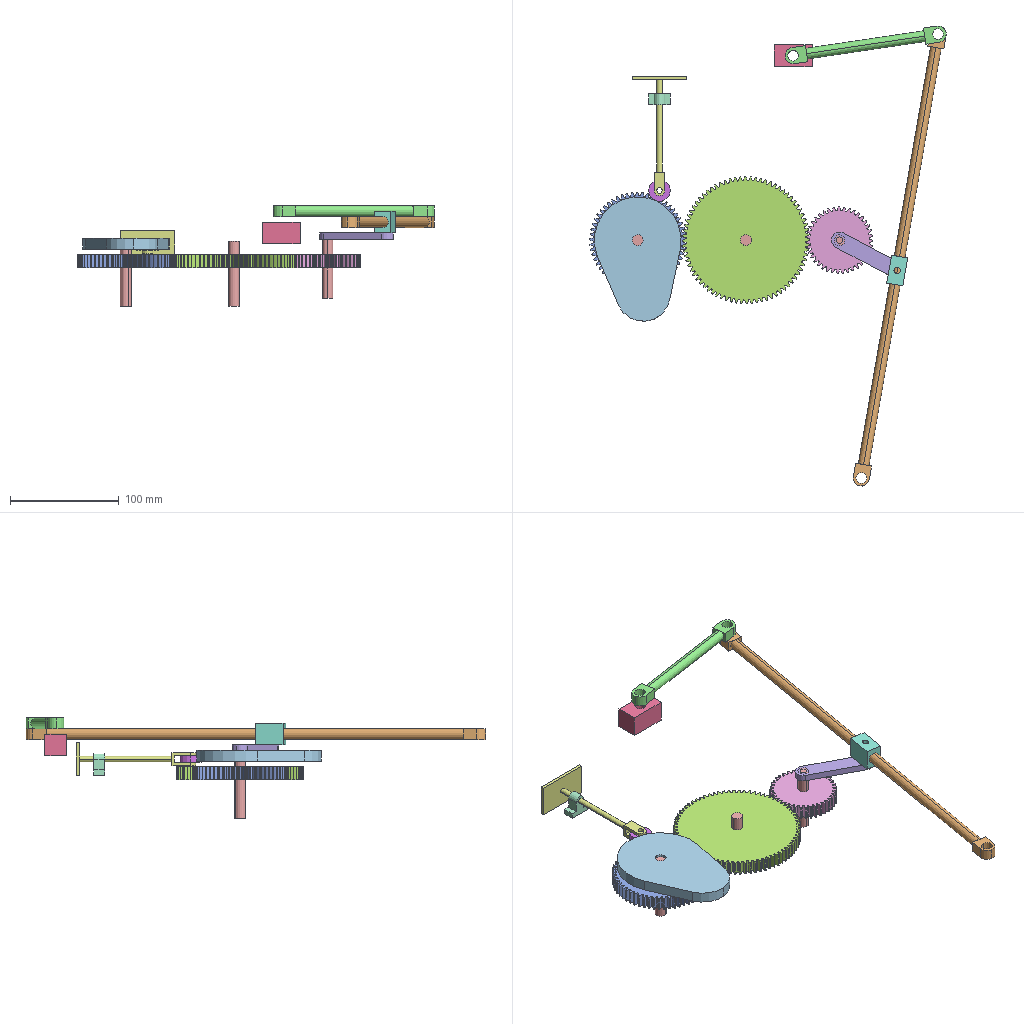Assembly | SolidWorks | 15 different items | 17 placed | box 329 x 424 x 93 mm
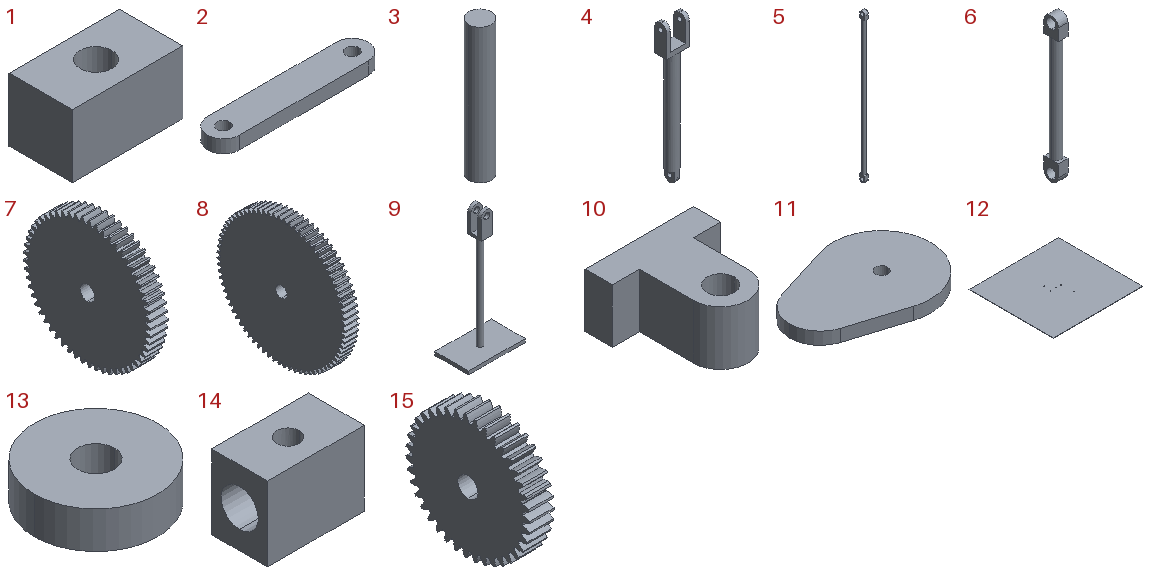Parts list (item | quantity | size | volume | features):
1 | x1 | 35 x 20 x 20 mm | 12429 mm3 | features Extrusion 1
2 | x1 | 75 x 15 x 6 mm | 6121 mm3 | features Extrusion 1
3 | x3 | 10 x 10 x 60 mm | 4712 mm3 | features Extrusion 1
4 | x1 | 30 x 16 x 188 mm | 32315 mm3 | features ICE 5, Extrusion 1
5 | x1 | 10 x 15 x 430 mm | 34577 mm3 | features ICE 3, Extrusion 1
6 | x1 | 10 x 15 x 150 mm | 12586 mm3 | features ICE 3, Extrusion 1
7 | x1 | 12 x 88.457 x 88.488 mm | 67194 mm3 | features Boss 3, Cut 3, CirPattern 2, Fillet 2, Revolution 1
8 | x1 | 12 x 116.937 x 116.937 mm | 120543 mm3 | features Boss 3, Cut 3, CirPattern 2, Fillet 2, Revolution 1
9 | x1 | 50 x 30 x 110 mm | 7427 mm3 | features ICE 4, Extrusion 1
10 | x1 | 20 x 20 x 10 mm | 2177 mm3 | features Extrusion 1, ICE 1
11 | x1 | 115 x 80 x 10 mm | 68139 mm3 | features Extrusion 1
12 | x1 | 1600 x 1500 x 5 mm | 11997688 mm3 | features Extrusion 1
13 | x1 | 20 x 20 x 6 mm | 1715 mm3 | features Extrusion 1
14 | x1 | 26 x 15 x 20 mm | 5462 mm3 | features Extrusion 1, ICE 1
15 | x1 | 12 x 61.434 x 61.481 mm | 30777 mm3 | features Boss 3, Cut 3, CirPattern 2, Fillet 2, Revolution 1
Mates (type | each side: item.copy, entity, surface, feature):
Concentric | 3.1 face cylinder Boss-Extrude1 | 7.1 face cylinder Bore
Concentric | 3.2 face cylinder Boss-Extrude1 | 8.1 face cylinder Bore
Concentric | 3.1 face cylinder Boss-Extrude1 | 12.1 face cylinder Boss-Extrude1
Concentric | 3.2 face cylinder Boss-Extrude1 | 12.1 face cylinder Boss-Extrude1
Parallel | 12.1 face plane Boss-Extrude1 | assembly plane
Coincident | 7.1 face plane Base-Revolve | 8.1 face plane Base-Revolve
Concentric | 12.1 face cylinder Boss-Extrude1 | 3.3 face cylinder Boss-Extrude1
Coincident | 3.1 face plane Boss-Extrude1 | 3.2 face plane Boss-Extrude1
Concentric | 3.3 face cylinder Boss-Extrude1 | 15.1 face cylinder Bore
Coincident | 8.1 face plane Base-Revolve | 15.1 face plane Base-Revolve
Coincident | 12.1 face plane Boss-Extrude1 | 3.3 face plane Boss-Extrude1 | 2 times
Concentric | 14.1 face cylinder Cut-Extrude1 | 5.1 face cylinder Boss-Extrude1
Concentric | 3.3 face cylinder Boss-Extrude1 | 2.1 face cylinder Boss-Extrude1
Concentric | 14.1 face cylinder Boss-Extrude1 | 2.1 face cylinder Boss-Extrude1
Coincident | 14.1 face plane Boss-Extrude1 | 2.1 face plane Boss-Extrude1
Coincident | 3.3 face plane Boss-Extrude1 | 2.1 face plane Boss-Extrude1
DistanceDim | 15.1 face plane Base-Revolve | 3.3 face plane Boss-Extrude1
Concentric | 12.1 face cylinder Boss-Extrude1 | 5.1 face cylinder Cut-Extrude1
Concentric | 5.1 face cylinder Cut-Extrude1 | 6.1 face cylinder Cut-Extrude1
Coincident | 5.1 face plane Boss-Extrude3 | 6.1 face plane Boss-Extrude3
Concentric | 6.1 face cylinder Cut-Extrude1 | 1.1 face cylinder Boss-Extrude1
DistanceDim | 1.1 face plane Boss-Extrude1 | 6.1 face plane Boss-Extrude2
GearDim | 15.1 face cylinder Base-Revolve | 8.1 face cylinder TeethCuts
GearDim | 8.1 face cylinder TeethCuts | 7.1 face cylinder Base-Revolve
Concentric | 3.1 face cylinder Boss-Extrude1 | 11.1 face cylinder Boss-Extrude1
DistanceDim | 11.1 face plane Boss-Extrude1 | 7.1 face plane Base-Revolve
Concentric | 9.1 face cylinder Cut-Extrude2 | 13.1 face cylinder Boss-Extrude1
Coincident | 9.1 face plane Cut-Extrude1 | 13.1 face plane Boss-Extrude1
DistanceDim | 13.1 face plane Boss-Extrude1 | 11.1 face plane Boss-Extrude1
Concentric | 9.1 face cylinder Boss-Extrude2 | 10.1 face cylinder Boss-Extrude1
CamTangent | 11.1 face plane Boss-Extrude1 | 13.1 face cylinder Boss-Extrude1
Concentric | 12.1 face cylinder Boss-Extrude1 | 10.1 face cylinder Cut-Extrude1
Parallel | 12.1 face plane Boss-Extrude1 | 10.1 face plane Boss-Extrude1
DistanceDim | 1.1 face plane Boss-Extrude1 | 12.1 face plane Boss-Extrude1